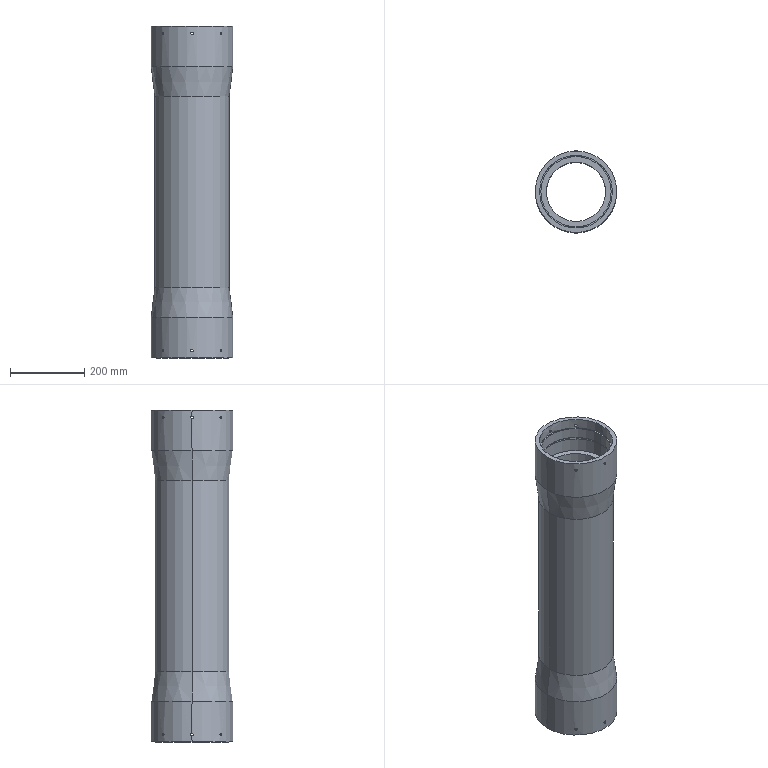Part | NX | features BREP 1 | 1 solid | 108 faces | box 220 x 220 x 895 mm | volume 10299409 mm3 | cylinder 72 | plane 16 | torus 12 | cone 8 | commonest cylinder face diameters 6.8 x32 196.752 x12 189.8 x8 200.752 x8 190 x4 220 x4